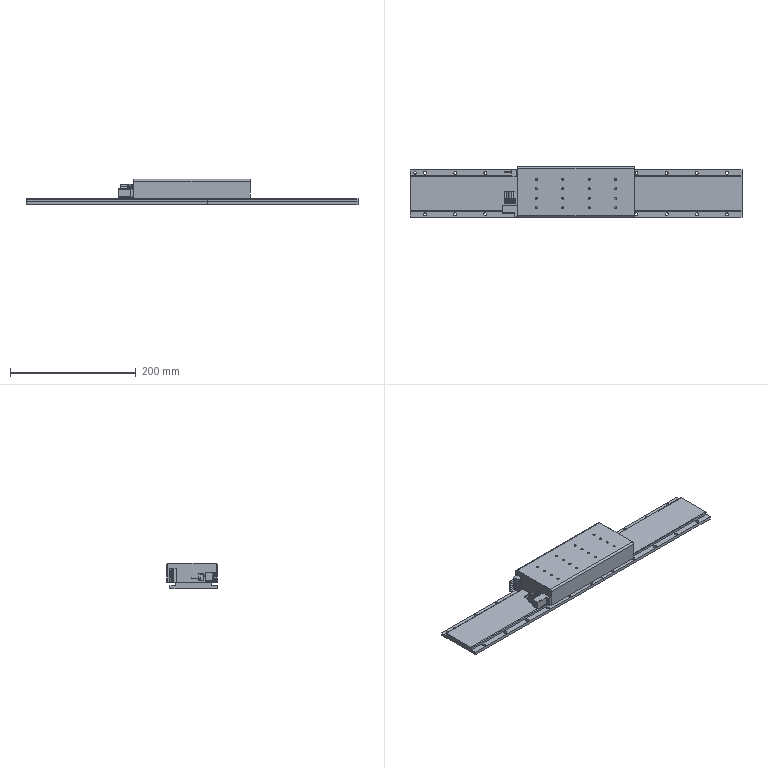Part | NX | features BREP 12 | 12 solids | 830 faces | box 527.8 x 80 x 40 mm | volume 773171 mm3 | plane 563 | cylinder 195 | cone 72 | commonest cylinder face diameters 4.8 x44 3.242 x32 1.404 x22 2.01 x22 2.8 x22 0.5 x12